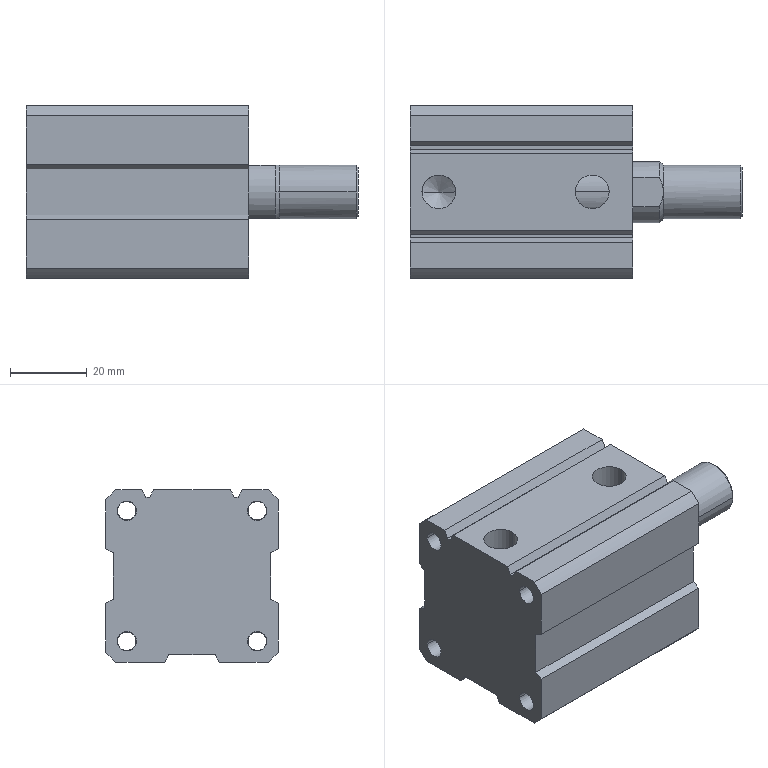Part | STEP file | Cylinder CDQ2A-32×20-DM Retract | 2 solids | 93 faces | box 86.5 x 45 x 45 mm | volume 118122 mm3 | cylinder 36 | plane 32 | cone 25 | commonest cylinder face diameters 5 x16 4.8 x8 8.8 x4 60 x4 14 x2 16 x2